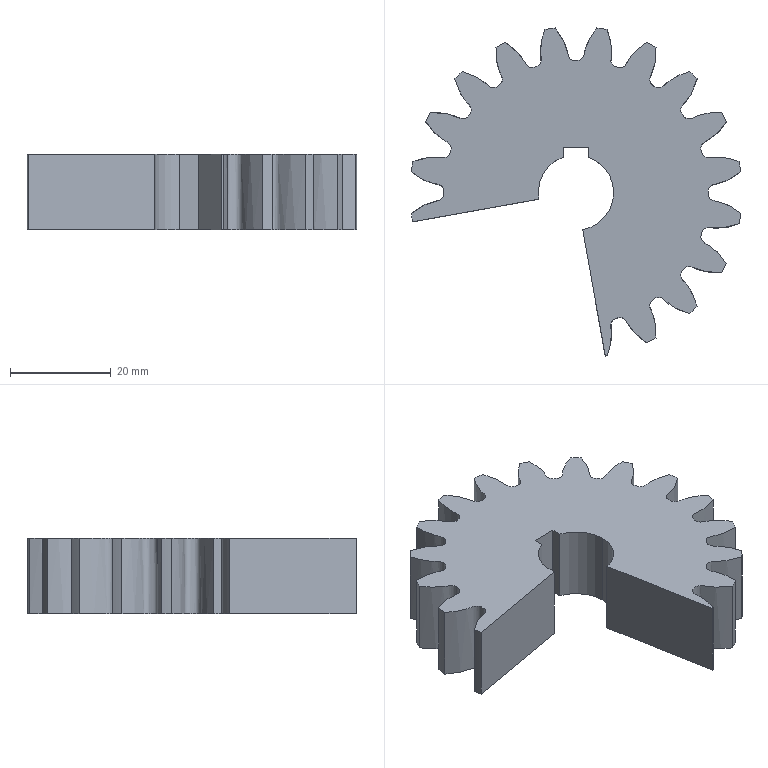Part | STEP file | Cuon T phu H01_5_Spur01 | 1 solid | 41 faces | box 65.481 x 65.224 x 15 mm | volume 29472 mm3 | cylinder 19 | spline 15 | plane 7 | commonest cylinder face diameters 66 x16 15 x3